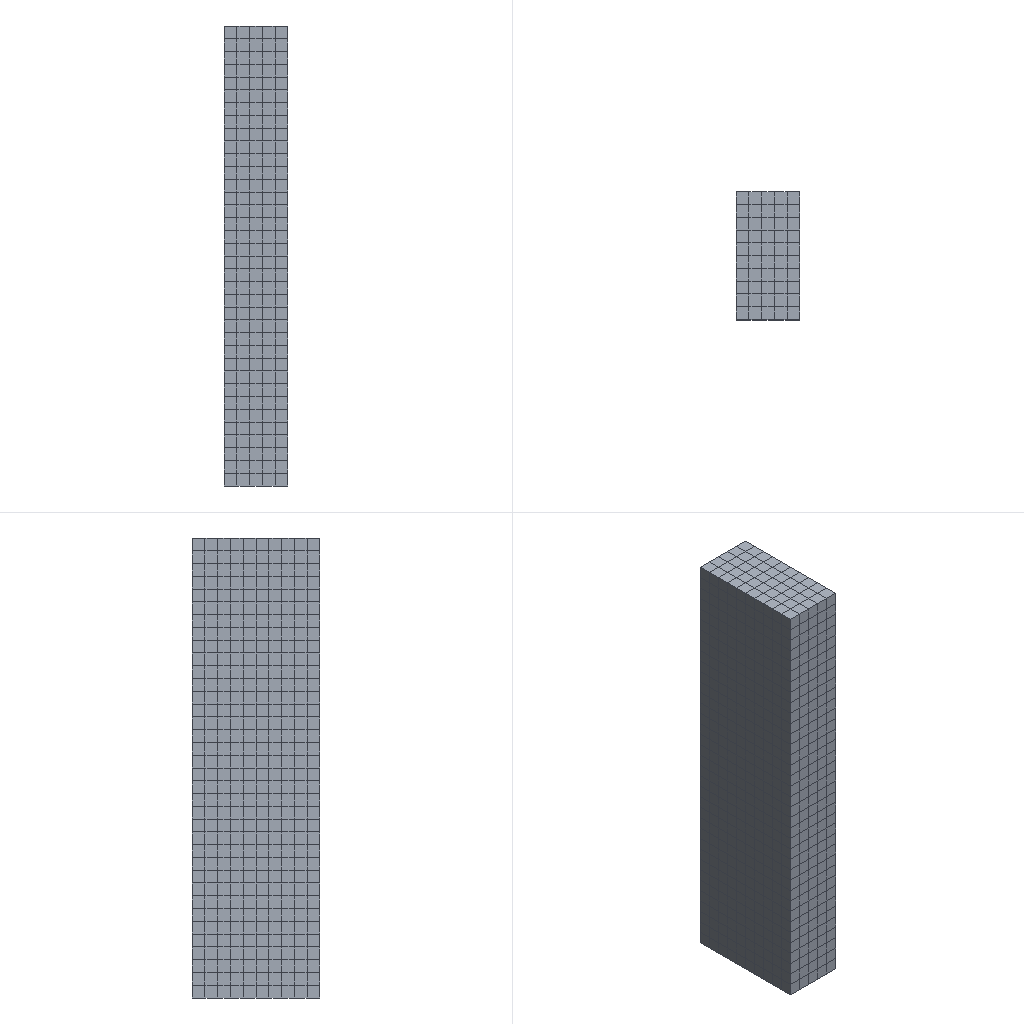Simulation study | abaqus
Set-up summary:
category,name,step,type,value,unit,region
solver,abaqus,,Abaqus/CAE 2024
units,mm-N-s-tonne (MPa),,inferred,E=30000 density=
analysis,Step-1,,static,nlgeom=True; time_period=1
mesh,nodes,,,3554
mesh,elements,,,2996
element_type,C3D8R,,,1800
element_type,T3D2,,,1196
material,con,,E,30000
material,con,,nu,0.2
material,con,,behaviors,plastic; concrete damaged plasticity; concrete compression hardening; concrete tension stiffening; concrete compression damage; concrete tension damage
material,d8,,E,210000
material,d8,,nu,0.3
material,d8,,yield,235
material,d8,,behaviors,plastic
material,d18,,E,210000
material,d18,,nu,0.3
material,d18,,yield,583
material,d18,,behaviors,plastic
section,con,,solid section,,,_PickedSet2
section,d18,,solid section,,,_PickedSet2_#7
section,d8,,solid section,,,_PickedSet2_#8
load,Load-3,Step-1,concentrated force,"10000 [dir=(0, -1, 0)]",,_PickedSet136
bc,BC-1,initial,fixed,"[dofs=rx,ry,rz,x,y,z n=6]",,Set-4
bc,BC-2,Step-1,fixed,"[dofs=ry,rz,x n=3]",,_PickedSet137
constraint,embedded element,,,1
constraint,coupling,,,1
Abaqus input file, long lists of numbers shortened:
*Heading
** Job name: deck Model name: Model-1
** Generated by: Abaqus/CAE 2024
*Preprint, echo=NO, model=NO, history=NO, contact=NO
**
** PARTS
**
*Part, name=con
*Node
      1,      -233.75,       -16.25,        1800.
      2,      -233.75,        33.75,        1800.
** (2440 more lines like these left out)
*Element, type=C3D8R
   1,  408,  409,  420,  419,    1,    2,   13,   12
   2,  409,  410,  421,  420,    2,    3,   14,   13
** (1798 more lines like these left out)
*Nset, nset=_PickedSet2, internal, generate
    1,  2442,     1
*Elset, elset=_PickedSet2, internal, generate
    1,  1800,     1
** Section: con
*Solid Section, elset=_PickedSet2, material=con
,
*End Part
**
*Part, name=gangjinlong
*Node
      1,       734.25,       393.75,     1753.125
      2,       734.25,       393.75,     1728.125
** (1109 more lines like these left out)
*Element, type=T3D2
1, 1, 2
2,   2, 101
** (1194 more lines like these left out)
*Nset, nset=_PickedSet2_#7, internal
    1,    2,    3,    4,    5,    6,    7,    8,    9,   10,   11,   12,   13,   14,   15,   16
   17,   18,   19,   20,   21,   22,   23,   24,   25,   26,   27,   28,   29,   30,   31,   32
** (21 more lines like these left out)
*Elset, elset=_PickedSet2_#7, internal
    1,    2,    3,    4,    5,    6,    7,    8,    9,   10,   11,   12,   13,   14,   15,   16
   17,   18,   19,   20,   21,   22,   23,   24,   25,   26,   27,   28,   29,   30,   31,   32
** (20 more lines like these left out)
*Nset, nset=_PickedSet2_#8, internal
    2,    3,    4,    5,    6,    7,    8,    9,   10,   11,   12,   13,   14,   15,   16,   17
   18,   19,   21,   22,   24,   25,   26,   27,   28,   29,   30,   31,   32,   33,   34,   35
** (51 more lines like these left out)
*Elset, elset=_PickedSet2_#8, internal
   71,   72,   73,   74,   75,   76,   78,   79,   80,   81,   82,   83,   88,   89,   90,   91
   92,   93,   94,   95,   96,   97,   98,   99,  100,  101,  102,  103,  104,  105,  106,  107
** (51 more lines like these left out)
** Section: d12
*Solid Section, elset=_PickedSet2_#7, material=d18
254.34,
** Section: d8
*Solid Section, elset=_PickedSet2_#8, material=d8
50.24,
*End Part
**
**
** ASSEMBLY
**
*Assembly, name=Assembly
**
*Instance, name=con-1, part=con
*End Instance
**
*Instance, name=gangjinlong-1, part=gangjinlong
       -843.,          50.,       21.875
*End Instance
**
*Node
      1,      -108.75,       483.75,           0.
*Nset, nset=Set-4, instance=con-1
    1,    2,    3,    4,    5,    6,    7,    8,    9,   10,   11,  408,  409,  410,  411,  412
  413,  414,  415,  416,  417,  418,  815,  816,  817,  818,  819,  820,  821,  822,  823,  824
** (3 more lines like these left out)
*Elset, elset=Set-4, instance=con-1
    1,    2,    3,    4,    5,    6,    7,    8,    9,   10,  361,  362,  363,  364,  365,  366
  367,  368,  369,  370,  721,  722,  723,  724,  725,  726,  727,  728,  729,  730, 1081, 1082
** (2 more lines like these left out)
*Nset, nset=m_Set-4, instance=gangjinlong-1, generate
    1,  1111,     1
*Elset, elset=m_Set-4, instance=gangjinlong-1, generate
    1,  1196,     1
*Nset, nset=_PickedSet134, internal, instance=con-1, generate
  407,  2442,   407
*Elset, elset=_PickedSet134, internal, instance=con-1, generate
  360,  1800,   360
*Nset, nset=_PickedSet135, internal
 1,
*Nset, nset=_PickedSet136, internal
 1,
*Nset, nset=_PickedSet137, internal
 1,
*Elset, elset=_Surf-2_S4, internal, instance=con-1, generate
   10,  1800,    10
*Surface, type=ELEMENT, name=Surf-2
_Surf-2_S4, S4
*Surface, type=NODE, name=_PickedSet134_CNS_, internal
_PickedSet134, 1.
** Constraint: Constraint-1
*Embedded Element
m_Set-4
** Constraint: Constraint-2
*Coupling, constraint name=Constraint-2, ref node=_PickedSet135, surface=_PickedSet134_CNS_
*Kinematic
*End Assembly
*Amplitude, name=Amp-1
             0.,              0.,              1.,              1.
**
** MATERIALS
**
*Material, name=con
*Elastic
30000., 0.2
*Concrete Damaged Plasticity
30.,    0.1,   1.16, 0.6667, 0.0005
*Concrete Compression Hardening
 10.88,         0.
 13.79,  8.889e-05
 14.414, 0.0001047
 15.365, 0.000134
 16.946, 0.0002035
 19.576, 0.0004826
 20.13, 0.0007944
 19.996, 0.0009457
 19.644, 0.001104
 19.144, 0.001268
 18.55, 0.001435
  17.905, 0.001603
 17.237, 0.001772
 16.567,  0.001942
 15.909, 0.002111
 15.271, 0.002279
 14.659, 0.002446
 14.076, 0.002612
 13.523, 0.002777
 13., 0.002942
 12.507, 0.003105
 12.041, 0.003267
 11.603, 0.003428
 11.191, 0.003589
 10.803, 0.003748
 10.437, 0.003907
 10.091, 0.004065
 9.459, 0.004379
 8.894, 0.004691
 8.387, 0.005001
  7.932, 0.005308
 7.52, 0.005615
 7.147, 0.00592
  6.808, 0.006224
 6.498, 0.006526
 6.214, 0.006828
 5.953,  0.007129
*Concrete Tension Stiffening
  2.058,         0.
  1.921,  1.841e-05
  1.716,  3.908e-05
  1.528,  5.921e-05
  1.37,  7.834e-05
  1.239,  9.654e-05
  1.131, 0.000114
  1.042, 0.0001308
 0.9662, 0.0001471
 0.9019, 0.0001631
 0.8466, 0.0001788
 0.6558, 0.0002542
 0.5431,  0.0003271
  0.4681, 0.0003987
 0.4141, 0.0004696
 0.3732,    0.00054
 0.341, 0.0006101
 0.3149, 0.0006801
 0.2932, 0.0007499
*Concrete Compression Damage
        0.,         0.
 0.05447,  8.889e-05
  0.06095, 0.0001047
 0.07232, 0.000134
  0.09691, 0.0002035
  0.1806, 0.0004826
  0.2607, 0.0007944
  0.2971, 0.0009457
   0.3344, 0.001104
  0.3719, 0.001268
  0.4087, 0.001435
   0.4445, 0.001603
  0.4789, 0.001772
    0.5116,  0.001942
   0.5425, 0.002111
   0.5715, 0.002279
  0.5986, 0.002446
  0.6239, 0.002612
  0.6473, 0.002777
  0.6691, 0.002942
  0.6893, 0.003105
  0.708, 0.003267
  0.7253, 0.003428
  0.7413, 0.003589
  0.7562, 0.003748
  0.7699, 0.003907
  0.7826, 0.004065
   0.8054, 0.004379
  0.825, 0.004691
  0.842, 0.005001
  0.8568, 0.005308
  0.8697, 0.005615
  0.881, 0.00592
  0.891, 0.006224
  0.8998, 0.006526
  0.9076, 0.006828
  0.9146,  0.007129
*Concrete Tension Damage
       0.,         0.
 0.2045,  1.841e-05
 0.379,  3.908e-05
 0.5095,  5.921e-05
  0.6053,  7.834e-05
 0.6762,  9.654e-05
 0.7298, 0.000114
 0.7709, 0.0001308
 0.8032, 0.0001471
 0.829, 0.0001631
 0.8499, 0.0001788
 0.9122, 0.0002542
 0.9417,  0.0003271
 0.958, 0.0003987
 0.9681, 0.0004696
 0.9749,    0.00054
 0.9796, 0.0006101
 0.983, 0.0006801
 0.9856, 0.0007499
*Material, name=d8
*Elastic
210000., 0.3
*Plastic
235.,   0.
400., 0.18
*Material, name=d18
*Elastic
210000., 0.3
*Plastic
583.,   0.
700., 0.18
**
** BOUNDARY CONDITIONS
**
** Name: BC-1 Type: Displacement/Rotation
*Boundary
Set-4, 1, 1
Set-4, 2, 2
Set-4, 3, 3
Set-4, 4, 4
Set-4, 5, 5
Set-4, 6, 6
** ----------------------------------------------------------------
**
** STEP: Step-1
**
*Step, name=Step-1, nlgeom=YES, inc=10000
*Static, stabilize=0.0002, allsdtol=0.05, continue=NO
0.01, 1., 1e-05, 0.1
**
** BOUNDARY CONDITIONS
**
** Name: BC-2 Type: Displacement/Rotation
*Boundary
_PickedSet137, 1, 1
_PickedSet137, 5, 5
_PickedSet137, 6, 6
**
** LOADS
**
** Name: Load-3   Type: Concentrated force
*Cload
_PickedSet136, 2, -10000.
**
** OUTPUT REQUESTS
**
*Restart, write, frequency=0
**
** FIELD OUTPUT: F-Output-1
**
*Output, field, variable=PRESELECT
**
** HISTORY OUTPUT: H-Output-1
**
*Output, history, variable=PRESELECT
*End Step
Results summary:
result,odb.job_status,,,JOB_STATUS_COMPLETED_SUCCESSFULLY,"consistent, unstated (Abaqus has no unit system)"
result,steps[0].procedure,Step-1,,*STATIC,"consistent, unstated (Abaqus has no unit system)"
result,steps[0].time_period,Step-1,,1,"consistent, unstated (Abaqus has no unit system)"
result,steps[0].n_frames,Step-1,,16,"consistent, unstated (Abaqus has no unit system)"
result,steps[0].last_frame.id,Step-1,,15,"consistent, unstated (Abaqus has no unit system)"
result,steps[0].last_frame.value,Step-1,,1,"consistent, unstated (Abaqus has no unit system)"
result,steps[0].last_frame.description,Step-1,,Increment     15: Step Time =    1.000,"consistent, unstated (Abaqus has no unit system)"
result,steps[0].completed,Step-1,,True,"consistent, unstated (Abaqus has no unit system)"
result,steps[0].max_U_magnitude,Step-1,,0.2491,"consistent, unstated (Abaqus has no unit system)"
result,steps[0].max_S_mises,Step-1,,9.959,"consistent, unstated (Abaqus has no unit system)"
result,steps[0].RF_sum[1],Step-1,,6.10352e-05,"consistent, unstated (Abaqus has no unit system)"
result,steps[0].RF_sum[2],Step-1,,9997.69,"consistent, unstated (Abaqus has no unit system)"
result,steps[0].RF_sum[3],Step-1,,0.0006104,"consistent, unstated (Abaqus has no unit system)"